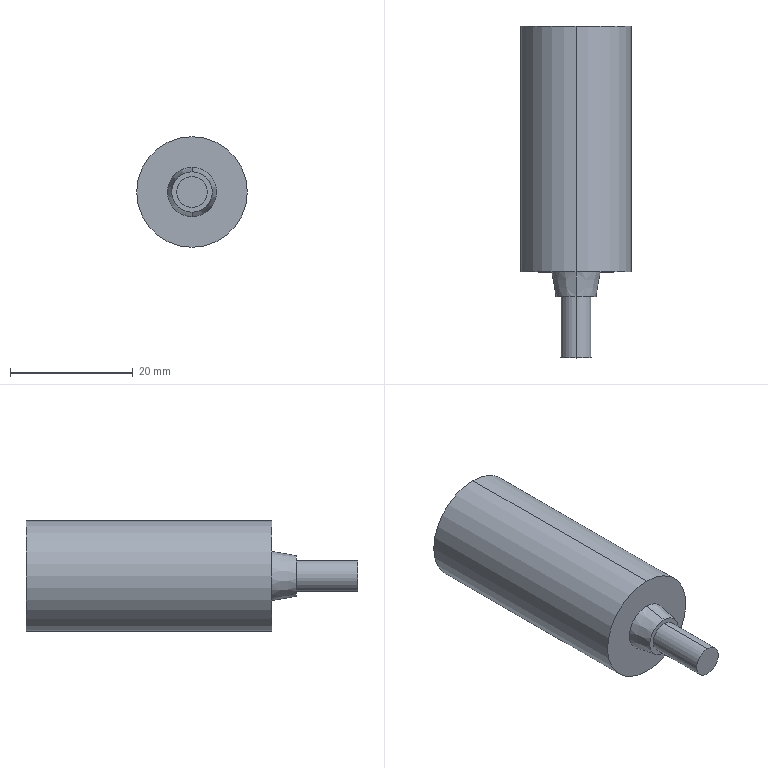Part | SolidWorks | features BaseBody 1 | 1 solid | 10 faces | box 18 x 54 x 18 mm | volume 10543 mm3 | cylinder 4 | plane 4 | cone 2 | commonest cylinder face diameters 5 x2 18 x2
STEP:
#1=CARTESIAN_POINT('',(137.047,1630.079,-1168.));
#2=VERTEX_POINT('',#1);
#3=CARTESIAN_POINT('',(137.047,1630.079,-1150.));
#4=VERTEX_POINT('',#3);
#5=CARTESIAN_POINT('',(137.047,1630.079,-1159.));
#6=DIRECTION('',(0.,-1.,0.));
#7=DIRECTION('',(0.,0.,-1.));
#8=AXIS2_PLACEMENT_3D('',#5,#6,#7);
#9=CIRCLE('',#8,9.);
#10=EDGE_CURVE('',#2,#4,#9,.T.);
#11=ORIENTED_EDGE('',*,*,#10,.T.);
#12=CARTESIAN_POINT('',(137.047,1590.079,-1150.));
#13=VERTEX_POINT('',#12);
#14=CARTESIAN_POINT('',(137.047,1630.079,-1150.));
#15=DIRECTION('',(0.,-1.,0.));
#16=VECTOR('',#15,1000.);
#17=LINE('',#14,#16);
#18=EDGE_CURVE('',#4,#13,#17,.T.);
#19=ORIENTED_EDGE('',*,*,#18,.T.);
#20=CARTESIAN_POINT('',(137.047,1590.079,-1168.));
#21=VERTEX_POINT('',#20);
#22=CARTESIAN_POINT('',(137.047,1590.079,-1159.));
#23=DIRECTION('',(0.,1.,0.));
#24=DIRECTION('',(0.,0.,-1.));
#25=AXIS2_PLACEMENT_3D('',#22,#23,#24);
#26=CIRCLE('',#25,9.);
#27=EDGE_CURVE('',#13,#21,#26,.T.);
#28=ORIENTED_EDGE('',*,*,#27,.T.);
#29=CARTESIAN_POINT('',(137.047,1630.079,-1168.));
#30=DIRECTION('',(0.,-1.,0.));
#31=VECTOR('',#30,1000.);
#32=LINE('',#29,#31);
#33=EDGE_CURVE('',#2,#21,#32,.T.);
#34=ORIENTED_EDGE('',*,*,#33,.F.);
#35=EDGE_LOOP('',(#11,#19,#28,#34));
#36=FACE_OUTER_BOUND('',#35,.T.);
#37=CARTESIAN_POINT('',(137.047,1630.079,-1159.));
#38=DIRECTION('',(0.,-1.,0.));
#39=DIRECTION('',(0.,0.,-1.));
#40=AXIS2_PLACEMENT_3D('',#37,#38,#39);
#41=CYLINDRICAL_SURFACE('',#40,9.);
#42=ADVANCED_FACE('',(#36),#41,.T.);
#43=CARTESIAN_POINT('',(137.047,1586.079,-1155.705));
#44=VERTEX_POINT('',#43);
#45=CARTESIAN_POINT('',(137.047,1586.079,-1162.295));
#46=VERTEX_POINT('',#45);
#47=CARTESIAN_POINT('',(137.047,1586.079,-1159.));
#48=DIRECTION('',(0.,1.,0.));
#49=DIRECTION('',(0.,0.,1.));
#50=AXIS2_PLACEMENT_3D('',#47,#48,#49);
#51=CIRCLE('',#50,3.295);
#52=EDGE_CURVE('',#44,#46,#51,.T.);
#53=ORIENTED_EDGE('',*,*,#52,.T.);
#54=CARTESIAN_POINT('',(137.047,1590.079,-1163.));
#55=VERTEX_POINT('',#54);
#56=CARTESIAN_POINT('',(137.047,1590.079,-1163.));
#57=DIRECTION('',(0.,0.9848,-0.1736));
#58=VECTOR('',#57,1000.);
#59=LINE('',#56,#58);
#60=EDGE_CURVE('',#46,#55,#59,.T.);
#61=ORIENTED_EDGE('',*,*,#60,.T.);
#62=CARTESIAN_POINT('',(137.047,1590.079,-1155.));
#63=VERTEX_POINT('',#62);
#64=CARTESIAN_POINT('',(137.047,1590.079,-1159.));
#65=DIRECTION('',(0.,-1.,0.));
#66=DIRECTION('',(0.,0.,1.));
#67=AXIS2_PLACEMENT_3D('',#64,#65,#66);
#68=CIRCLE('',#67,4.);
#69=EDGE_CURVE('',#55,#63,#68,.T.);
#70=ORIENTED_EDGE('',*,*,#69,.T.);
#71=CARTESIAN_POINT('',(137.047,1590.079,-1155.));
#72=DIRECTION('',(0.,0.9848,0.1736));
#73=VECTOR('',#72,1000.);
#74=LINE('',#71,#73);
#75=EDGE_CURVE('',#44,#63,#74,.T.);
#76=ORIENTED_EDGE('',*,*,#75,.F.);
#77=EDGE_LOOP('',(#53,#61,#70,#76));
#78=FACE_OUTER_BOUND('',#77,.T.);
#79=CARTESIAN_POINT('',(137.047,1590.079,-1159.));
#80=DIRECTION('',(0.,1.,0.));
#81=DIRECTION('',(0.,0.,1.));
#82=AXIS2_PLACEMENT_3D('',#79,#80,#81);
#83=CONICAL_SURFACE('',#82,4.,0.1745);
#84=ADVANCED_FACE('',(#78),#83,.T.);
#85=CARTESIAN_POINT('',(137.047,1576.079,-1156.5));
#86=VERTEX_POINT('',#85);
#87=CARTESIAN_POINT('',(137.047,1576.079,-1161.5));
#88=VERTEX_POINT('',#87);
#89=CARTESIAN_POINT('',(137.047,1576.079,-1159.));
#90=DIRECTION('',(0.,1.,0.));
#91=DIRECTION('',(0.,0.,1.));
#92=AXIS2_PLACEMENT_3D('',#89,#90,#91);
#93=CIRCLE('',#92,2.5);
#94=EDGE_CURVE('',#86,#88,#93,.T.);
#95=ORIENTED_EDGE('',*,*,#94,.T.);
#96=CARTESIAN_POINT('',(137.047,1586.079,-1161.5));
#97=VERTEX_POINT('',#96);
#98=CARTESIAN_POINT('',(137.047,1576.079,-1161.5));
#99=DIRECTION('',(0.,1.,0.));
#100=VECTOR('',#99,1000.);
#101=LINE('',#98,#100);
#102=EDGE_CURVE('',#88,#97,#101,.T.);
#103=ORIENTED_EDGE('',*,*,#102,.T.);
#104=CARTESIAN_POINT('',(137.047,1586.079,-1156.5));
#105=VERTEX_POINT('',#104);
#106=CARTESIAN_POINT('',(137.047,1586.079,-1159.));
#107=DIRECTION('',(0.,1.,0.));
#108=DIRECTION('',(0.,0.,1.));
#109=AXIS2_PLACEMENT_3D('',#106,#107,#108);
#110=CIRCLE('',#109,2.5);
#111=EDGE_CURVE('',#105,#97,#110,.T.);
#112=ORIENTED_EDGE('',*,*,#111,.F.);
#113=CARTESIAN_POINT('',(137.047,1576.079,-1156.5));
#114=DIRECTION('',(0.,1.,0.));
#115=VECTOR('',#114,1000.);
#116=LINE('',#113,#115);
#117=EDGE_CURVE('',#86,#105,#116,.T.);
#118=ORIENTED_EDGE('',*,*,#117,.F.);
#119=EDGE_LOOP('',(#95,#103,#112,#118));
#120=FACE_OUTER_BOUND('',#119,.T.);
#121=CARTESIAN_POINT('',(137.047,1576.079,-1159.));
#122=DIRECTION('',(0.,1.,0.));
#123=DIRECTION('',(0.,0.,1.));
#124=AXIS2_PLACEMENT_3D('',#121,#122,#123);
#125=CYLINDRICAL_SURFACE('',#124,2.5);
#126=ADVANCED_FACE('',(#120),#125,.T.);
#127=ORIENTED_EDGE('',*,*,#18,.F.);
#128=CARTESIAN_POINT('',(137.047,1630.079,-1159.));
#129=DIRECTION('',(0.,-1.,0.));
#130=DIRECTION('',(0.,0.,-1.));
#131=AXIS2_PLACEMENT_3D('',#128,#129,#130);
#132=CIRCLE('',#131,9.);
#133=EDGE_CURVE('',#4,#2,#132,.T.);
#134=ORIENTED_EDGE('',*,*,#133,.T.);
#135=ORIENTED_EDGE('',*,*,#33,.T.);
#136=CARTESIAN_POINT('',(137.047,1590.079,-1159.));
#137=DIRECTION('',(0.,1.,0.));
#138=DIRECTION('',(0.,0.,-1.));
#139=AXIS2_PLACEMENT_3D('',#136,#137,#138);
#140=CIRCLE('',#139,9.);
#141=EDGE_CURVE('',#21,#13,#140,.T.);
#142=ORIENTED_EDGE('',*,*,#141,.T.);
#143=EDGE_LOOP('',(#127,#134,#135,#142));
#144=FACE_OUTER_BOUND('',#143,.T.);
#145=CARTESIAN_POINT('',(137.047,1630.079,-1159.));
#146=DIRECTION('',(0.,-1.,0.));
#147=DIRECTION('',(0.,0.,-1.));
#148=AXIS2_PLACEMENT_3D('',#145,#146,#147);
#149=CYLINDRICAL_SURFACE('',#148,9.);
#150=ADVANCED_FACE('',(#144),#149,.T.);
#151=ORIENTED_EDGE('',*,*,#10,.F.);
#152=ORIENTED_EDGE('',*,*,#133,.F.);
#153=EDGE_LOOP('',(#151,#152));
#154=FACE_OUTER_BOUND('',#153,.T.);
#155=CARTESIAN_POINT('',(137.047,1630.079,-1159.));
#156=DIRECTION('',(0.,1.,0.));
#157=DIRECTION('',(0.,0.,1.));
#158=AXIS2_PLACEMENT_3D('',#155,#156,#157);
#159=PLANE('',#158);
#160=ADVANCED_FACE('',(#154),#159,.T.);
#161=CARTESIAN_POINT('',(137.047,1590.079,-1159.));
#162=DIRECTION('',(0.,-1.,0.));
#163=DIRECTION('',(0.,0.,1.));
#164=AXIS2_PLACEMENT_3D('',#161,#162,#163);
#165=CIRCLE('',#164,4.);
#166=EDGE_CURVE('',#63,#55,#165,.T.);
#167=ORIENTED_EDGE('',*,*,#166,.F.);
#168=ORIENTED_EDGE('',*,*,#69,.F.);
#169=EDGE_LOOP('',(#167,#168));
#170=FACE_BOUND('',#169,.T.);
#171=ORIENTED_EDGE('',*,*,#141,.F.);
#172=ORIENTED_EDGE('',*,*,#27,.F.);
#173=EDGE_LOOP('',(#171,#172));
#174=FACE_OUTER_BOUND('',#173,.T.);
#175=CARTESIAN_POINT('',(137.047,1590.079,-1159.));
#176=DIRECTION('',(0.,1.,0.));
#177=DIRECTION('',(0.,0.,1.));
#178=AXIS2_PLACEMENT_3D('',#175,#176,#177);
#179=PLANE('',#178);
#180=ADVANCED_FACE('',(#170,#174),#179,.F.);
#181=ORIENTED_EDGE('',*,*,#60,.F.);
#182=CARTESIAN_POINT('',(137.047,1586.079,-1159.));
#183=DIRECTION('',(0.,1.,0.));
#184=DIRECTION('',(0.,0.,1.));
#185=AXIS2_PLACEMENT_3D('',#182,#183,#184);
#186=CIRCLE('',#185,3.295);
#187=EDGE_CURVE('',#46,#44,#186,.T.);
#188=ORIENTED_EDGE('',*,*,#187,.T.);
#189=ORIENTED_EDGE('',*,*,#75,.T.);
#190=ORIENTED_EDGE('',*,*,#166,.T.);
#191=EDGE_LOOP('',(#181,#188,#189,#190));
#192=FACE_OUTER_BOUND('',#191,.T.);
#193=CARTESIAN_POINT('',(137.047,1590.079,-1159.));
#194=DIRECTION('',(0.,1.,0.));
#195=DIRECTION('',(0.,0.,1.));
#196=AXIS2_PLACEMENT_3D('',#193,#194,#195);
#197=CONICAL_SURFACE('',#196,4.,0.1745);
#198=ADVANCED_FACE('',(#192),#197,.T.);
#199=ORIENTED_EDGE('',*,*,#111,.T.);
#200=CARTESIAN_POINT('',(137.047,1586.079,-1159.));
#201=DIRECTION('',(0.,1.,0.));
#202=DIRECTION('',(0.,0.,1.));
#203=AXIS2_PLACEMENT_3D('',#200,#201,#202);
#204=CIRCLE('',#203,2.5);
#205=EDGE_CURVE('',#97,#105,#204,.T.);
#206=ORIENTED_EDGE('',*,*,#205,.T.);
#207=EDGE_LOOP('',(#199,#206));
#208=FACE_BOUND('',#207,.T.);
#209=ORIENTED_EDGE('',*,*,#52,.F.);
#210=ORIENTED_EDGE('',*,*,#187,.F.);
#211=EDGE_LOOP('',(#209,#210));
#212=FACE_OUTER_BOUND('',#211,.T.);
#213=CARTESIAN_POINT('',(137.047,1586.079,-1159.));
#214=DIRECTION('',(0.,-1.,0.));
#215=DIRECTION('',(0.,0.,-1.));
#216=AXIS2_PLACEMENT_3D('',#213,#214,#215);
#217=PLANE('',#216);
#218=ADVANCED_FACE('',(#208,#212),#217,.T.);
#219=ORIENTED_EDGE('',*,*,#102,.F.);
#220=CARTESIAN_POINT('',(137.047,1576.079,-1159.));
#221=DIRECTION('',(0.,1.,0.));
#222=DIRECTION('',(0.,0.,1.));
#223=AXIS2_PLACEMENT_3D('',#220,#221,#222);
#224=CIRCLE('',#223,2.5);
#225=EDGE_CURVE('',#88,#86,#224,.T.);
#226=ORIENTED_EDGE('',*,*,#225,.T.);
#227=ORIENTED_EDGE('',*,*,#117,.T.);
#228=ORIENTED_EDGE('',*,*,#205,.F.);
#229=EDGE_LOOP('',(#219,#226,#227,#228));
#230=FACE_OUTER_BOUND('',#229,.T.);
#231=CARTESIAN_POINT('',(137.047,1576.079,-1159.));
#232=DIRECTION('',(0.,1.,0.));
#233=DIRECTION('',(0.,0.,1.));
#234=AXIS2_PLACEMENT_3D('',#231,#232,#233);
#235=CYLINDRICAL_SURFACE('',#234,2.5);
#236=ADVANCED_FACE('',(#230),#235,.T.);
#237=ORIENTED_EDGE('',*,*,#94,.F.);
#238=ORIENTED_EDGE('',*,*,#225,.F.);
#239=EDGE_LOOP('',(#237,#238));
#240=FACE_OUTER_BOUND('',#239,.T.);
#241=CARTESIAN_POINT('',(137.047,1576.079,-1159.));
#242=DIRECTION('',(0.,-1.,0.));
#243=DIRECTION('',(0.,0.,-1.));
#244=AXIS2_PLACEMENT_3D('',#241,#242,#243);
#245=PLANE('',#244);
#246=ADVANCED_FACE('',(#240),#245,.T.);
#247=CLOSED_SHELL('',(#42,#84,#126,#150,#160,#180,#198,#218,#236,#246));
#248=MANIFOLD_SOLID_BREP('',#247);
#249=CARTESIAN_POINT('',(0.,0.,0.));
#250=DIRECTION('',(0.,0.,1.));
#251=DIRECTION('',(1.,0.,0.));
#252=AXIS2_PLACEMENT_3D('',#249,#250,#251);
#253=(LENGTH_UNIT()NAMED_UNIT(*)SI_UNIT(.MILLI.,.METRE.));
#254=UNCERTAINTY_MEASURE_WITH_UNIT(LENGTH_MEASURE(0.00001),#253,'','');
#255=(NAMED_UNIT(*)PLANE_ANGLE_UNIT()SI_UNIT($,.RADIAN.));
#256=(NAMED_UNIT(*)SI_UNIT($,.STERADIAN.)SOLID_ANGLE_UNIT());
#257=(GEOMETRIC_REPRESENTATION_CONTEXT(3)GLOBAL_UNCERTAINTY_ASSIGNED_CONTEXT((#254))GLOBAL_UNIT_ASSIGNED_CONTEXT((#253,#255,#256))REPRESENTATION_CONTEXT('',''));
#258=ADVANCED_BREP_SHAPE_REPRESENTATION('',(#248,#252),#257);